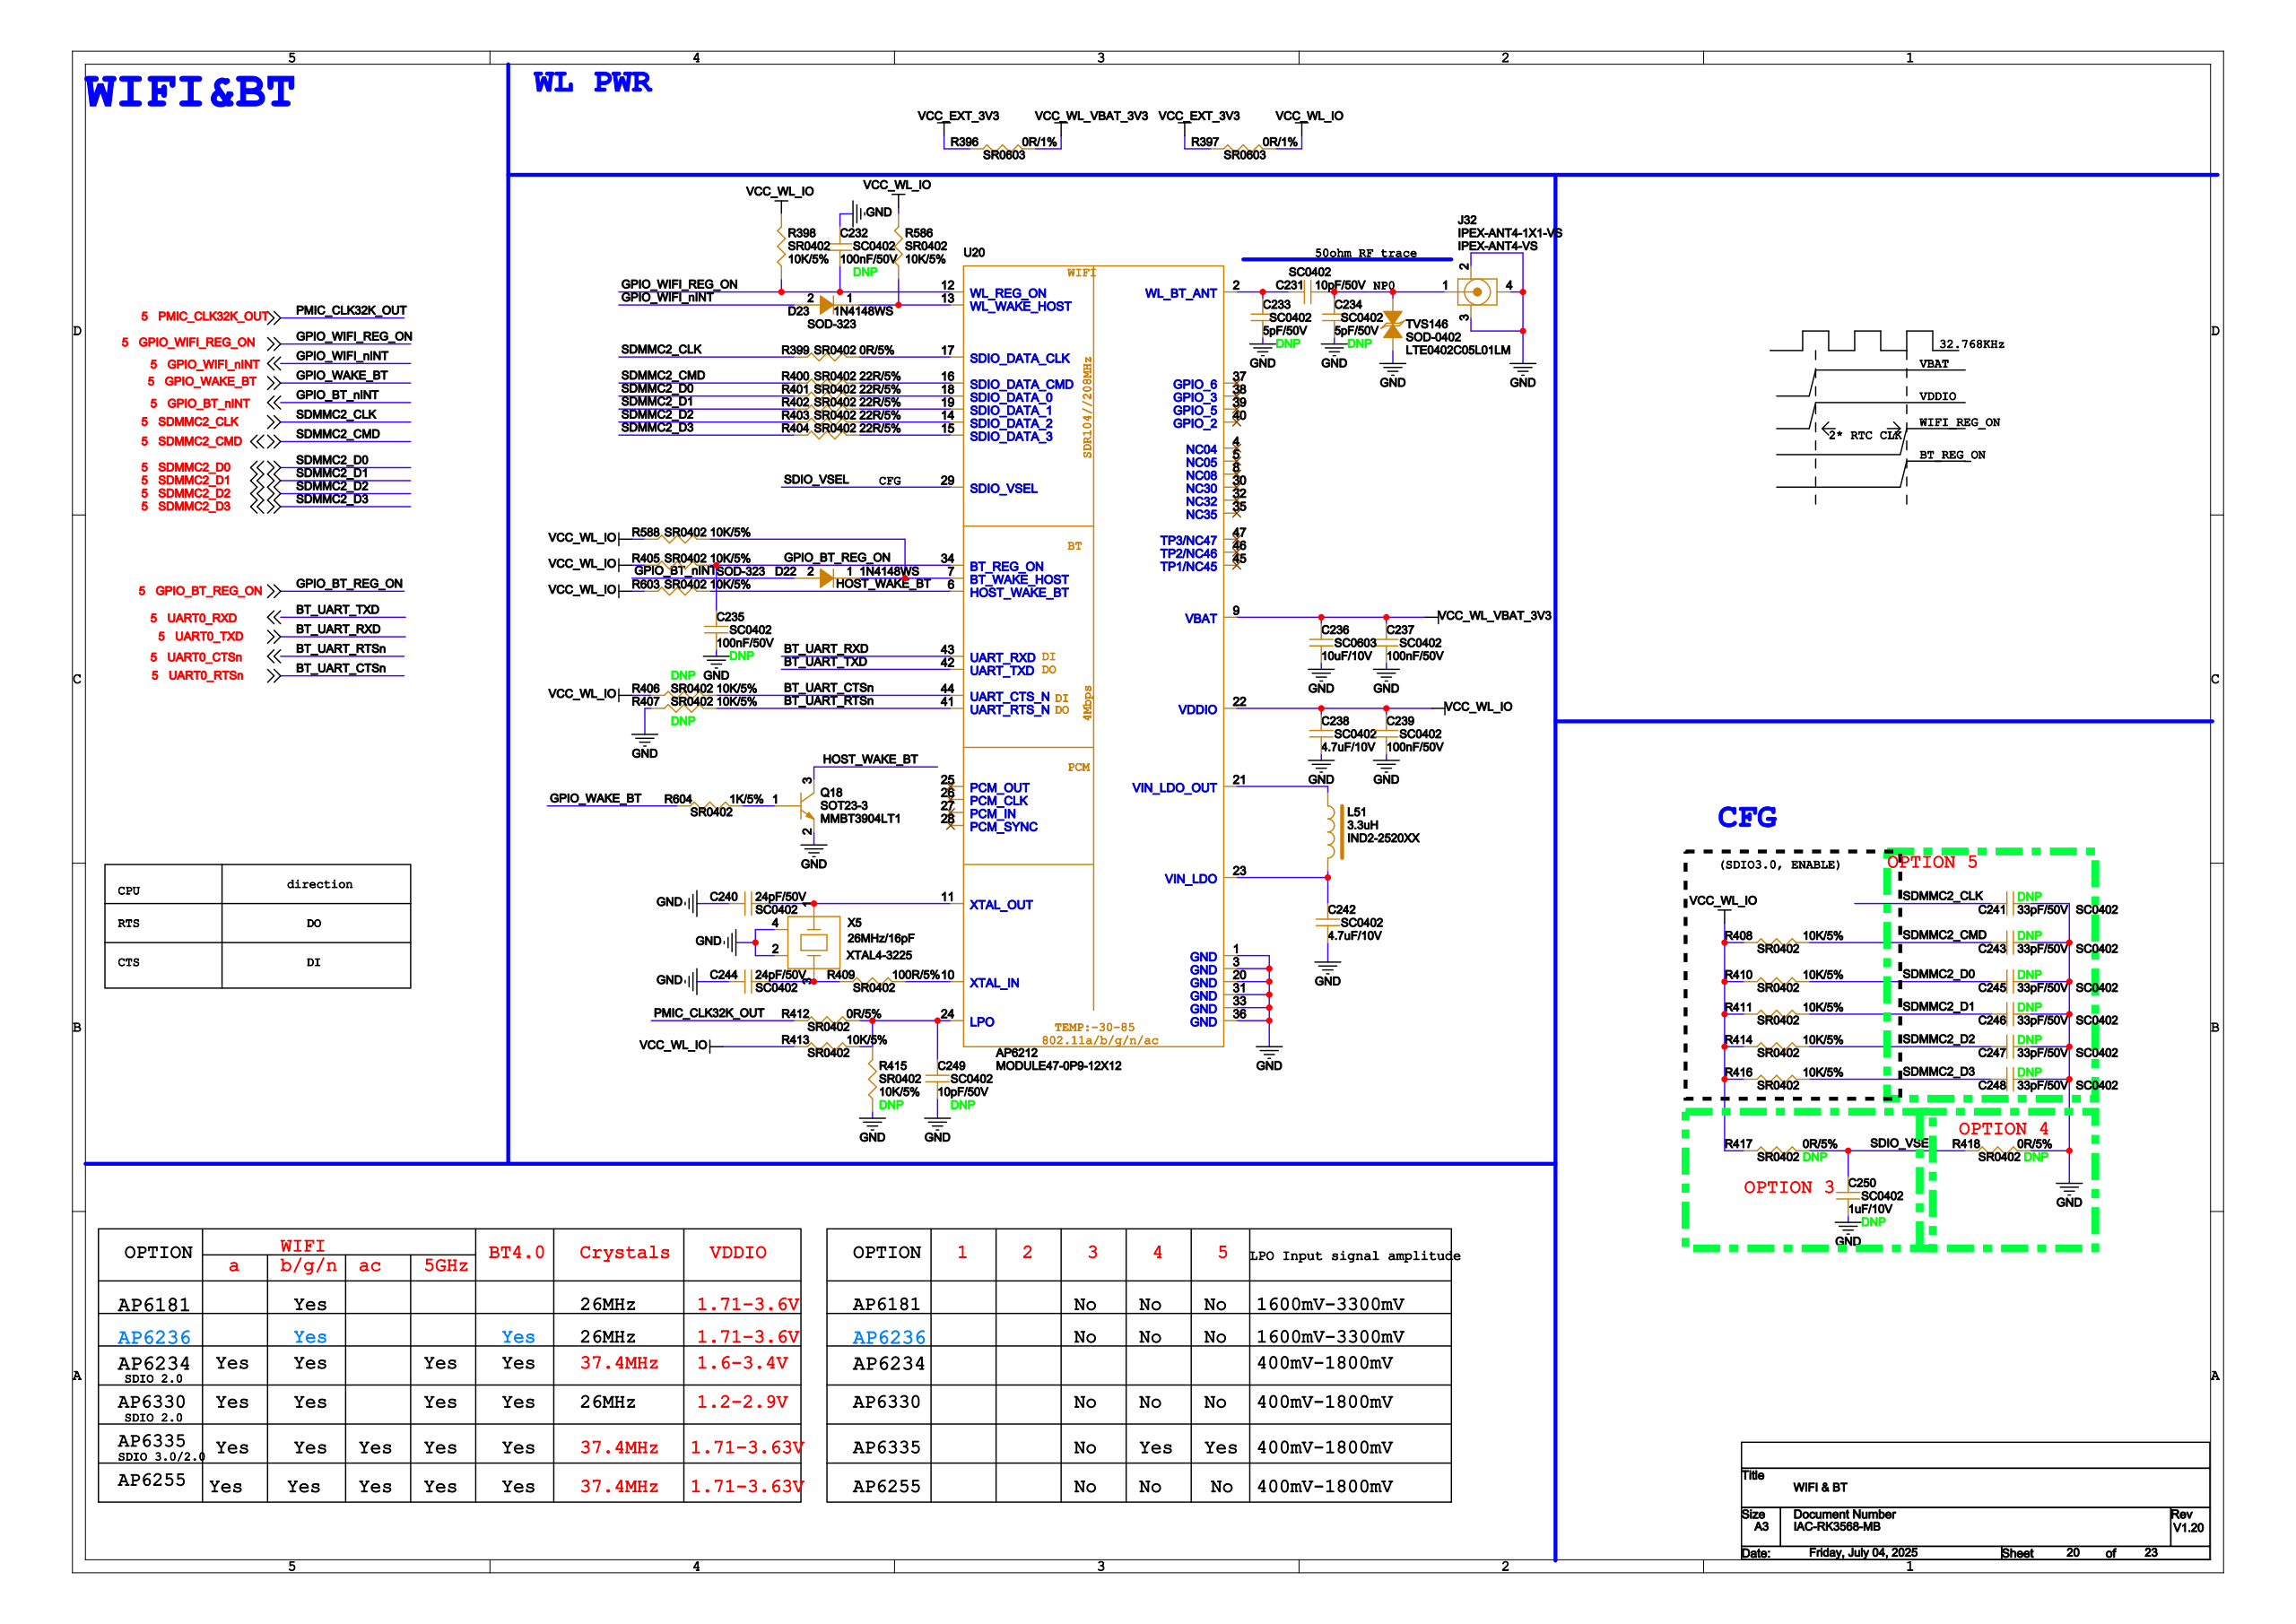Circuit board | Cadence Allegro | 1138 parts | 722 nets | one sheet of the schematic
Parts on this sheet (reference | value | footprint):
C231 | 10pF/50V | SC0402
C232 | 100nF/50V | SC0402
C233 | 5pF/50V | SC0402
C234 | 5pF/50V | SC0402
C235 | 100nF/50V | SC0402
C236 | 10uF/10V | SC0603
C237 | 100nF/50V | SC0402
C238 | 4.7uF/10V | SC0402
C239 | 100nF/50V | SC0402
C240 | 24pF/50V | SC0402
C241 | 33pF/50V | SC0402
C242 | 4.7uF/10V | SC0402
C243 | 33pF/50V | SC0402
C244 | 24pF/50V | SC0402
C245 | 33pF/50V | SC0402
C246 | 33pF/50V | SC0402
C247 | 33pF/50V | SC0402
C248 | 33pF/50V | SC0402
C249 | 10pF/50V | SC0402
C250 | 1uF/10V | SC0402
D22 | 1N4148WS | SOD-323
D23 | 1N4148WS | SOD-323
J32 | IPEX-ANT4-1X1-VS | IPEX-ANT4-VS
L51 | 3.3uH | IND2-2520XX
Q18 | MMBT3904LT1 | SOT23-3
R396 | 0R/1% | SR0603
R397 | 0R/1% | SR0603
R398 | 10K/5% | SR0402
R399 | 0R/5% | SR0402
R400 | 22R/5% | SR0402
R401 | 22R/5% | SR0402
R402 | 22R/5% | SR0402
R403 | 22R/5% | SR0402
R404 | 22R/5% | SR0402
R405 | 10K/5% | SR0402
R406 | 10K/5% | SR0402
R407 | 10K/5% | SR0402
R408 | 10K/5% | SR0402
R409 | 100R/5% | SR0402
R410 | 10K/5% | SR0402
R411 | 10K/5% | SR0402
R412 | 0R/5% | SR0402
R413 | 10K/5% | SR0402
R414 | 10K/5% | SR0402
R415 | 10K/5% | SR0402
R416 | 10K/5% | SR0402
R417 | 0R/5% | SR0402
R418 | 0R/5% | SR0402
R586 | 10K/5% | SR0402
R588 | 10K/5% | SR0402
R603 | 10K/5% | SR0402
R604 | 1K/5% | SR0402
TVS146 | LTE0402C05L01LM | SOD-0402
U20 | AP6212 | MODULE47-0P9-12X12
X5 | 26MHz/16pF | XTAL4-3225
Nets of these parts (net: part-pin ...):
VCC_EXT_3V3: R396-1 R397-1
GND: C232-2 C233-2 C234-2 C235-2 C236-2 C237-2 C238-2 C239-2 C240-1 C241-2 C242-2 C243-2 C244-1 C245-2 C246-2 C247-2 C248-2 C249-2 C250-2 J32-2 J32-3 J32-4 Q18-2 R407-1 R415-1 R418-2 TVS146-1 X5-2 X5-4 U20-1 U20-3 U20-20 U20-31 U20-33 U20-36
N7276856: Q18-1 R604-2
HOST_WAKE_BT: Q18-3 R603-2 U20-6
VCC_WL_VBAT_3V3: C236-1 C237-1 R396-2 U20-9
SDIO_VSEL: C250-1 R417-2 R418-1 U20-29
N19639563: C231-1 C233-1 U20-2
N19639556: C231-2 C234-1 J32-1 TVS146-2
N197936: C249-1 R412-2 R413-2 R415-2 U20-24
N19639705: C240-2 X5-1 U20-11
N19639707: C244-2 R409-1 X5-3
SDMMC2_CLK: C241-1 R399-1
SDMMC2_CMD: C243-1 R400-1 R408-2
SDMMC2_D0: C245-1 R401-1 R410-2
SDMMC2_D1: C246-1 R402-1 R411-2
SDMMC2_D2: C247-1 R403-1 R414-2
SDMMC2_D3: C248-1 R404-1 R416-2
N19639722: L51-1 U20-21
N19639726: C242-1 L51-2 U20-23
N19639452: R409-2 U20-10
GPIO_BT_REG_ON: C235-1 R405-2 U20-34
UART0_CTSN: R407-2 U20-41
UART0_RTSN: R406-2 U20-44
UART0_RXD: U20-42
UART0_TXD: U20-43
GPIO_WIFI_REG_ON: C232-1 R398-1 U20-12
GPIO_BT_NINT: D22-2
GPIO_WIFI_NINT: D23-2
GPIO_WAKE_BT: R604-1
PMIC_CLK32K_OUT: R412-1
N5444852: D22-1 R588-2 U20-7
N3598879: R401-2 U20-18
N3598923: R402-2 U20-19
N3598967: R403-2 U20-14
N3599011: R404-2 U20-15
N19639775: R399-2 U20-17
N3598835: R400-2 U20-16
VCC_WL_IO: C238-1 C239-1 R397-2 R398-2 R405-1 R406-1 R408-1 R410-1 R411-1 R413-1 R414-1 R416-1 R417-1 R586-2 R588-1 R603-1 U20-22
N5441939: D23-1 R586-1 U20-13